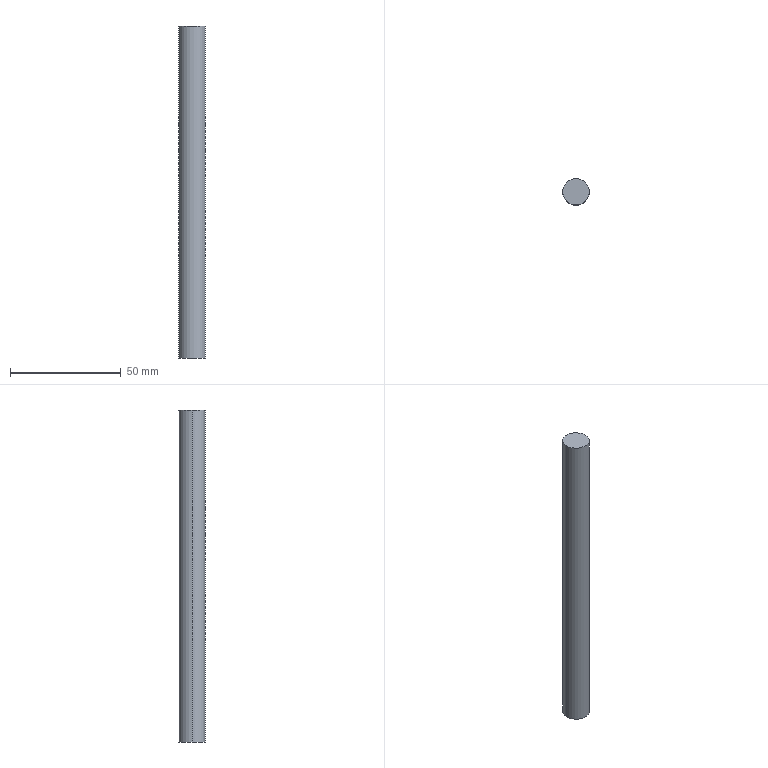Part | SolidWorks | features Extrusion 1 | 1 solid | 4 faces | box 12 x 12 x 150 mm | volume 16965 mm3 | cylinder 2 | plane 2 | commonest cylinder face diameters 12 x2
STEP:
#1=CARTESIAN_POINT('',(6.,0.,75.));
#2=VERTEX_POINT('',#1);
#3=CARTESIAN_POINT('',(-6.,0.,75.));
#4=VERTEX_POINT('',#3);
#5=CARTESIAN_POINT('',(0.,0.,75.));
#6=DIRECTION('',(0.,0.,1.));
#7=DIRECTION('',(1.,0.,0.));
#8=AXIS2_PLACEMENT_3D('',#5,#6,#7);
#9=CIRCLE('',#8,6.);
#10=EDGE_CURVE('',#2,#4,#9,.T.);
#11=ORIENTED_EDGE('',*,*,#10,.F.);
#12=CARTESIAN_POINT('',(6.,0.,-75.));
#13=VERTEX_POINT('',#12);
#14=CARTESIAN_POINT('',(6.,0.,75.));
#15=DIRECTION('',(0.,0.,-1.));
#16=VECTOR('',#15,1000.);
#17=LINE('',#14,#16);
#18=EDGE_CURVE('',#2,#13,#17,.T.);
#19=ORIENTED_EDGE('',*,*,#18,.T.);
#20=CARTESIAN_POINT('',(-6.,0.,-75.));
#21=VERTEX_POINT('',#20);
#22=CARTESIAN_POINT('',(0.,0.,-75.));
#23=DIRECTION('',(0.,0.,1.));
#24=DIRECTION('',(1.,0.,0.));
#25=AXIS2_PLACEMENT_3D('',#22,#23,#24);
#26=CIRCLE('',#25,6.);
#27=EDGE_CURVE('',#13,#21,#26,.T.);
#28=ORIENTED_EDGE('',*,*,#27,.T.);
#29=CARTESIAN_POINT('',(-6.,0.,75.));
#30=DIRECTION('',(0.,0.,-1.));
#31=VECTOR('',#30,1000.);
#32=LINE('',#29,#31);
#33=EDGE_CURVE('',#4,#21,#32,.T.);
#34=ORIENTED_EDGE('',*,*,#33,.F.);
#35=EDGE_LOOP('',(#11,#19,#28,#34));
#36=FACE_OUTER_BOUND('',#35,.T.);
#37=CARTESIAN_POINT('',(0.,0.,75.));
#38=DIRECTION('',(0.,0.,-1.));
#39=DIRECTION('',(-1.,0.,0.));
#40=AXIS2_PLACEMENT_3D('',#37,#38,#39);
#41=CYLINDRICAL_SURFACE('',#40,6.);
#42=ADVANCED_FACE('',(#36),#41,.T.);
#43=ORIENTED_EDGE('',*,*,#18,.F.);
#44=CARTESIAN_POINT('',(0.,0.,75.));
#45=DIRECTION('',(0.,0.,1.));
#46=DIRECTION('',(1.,0.,0.));
#47=AXIS2_PLACEMENT_3D('',#44,#45,#46);
#48=CIRCLE('',#47,6.);
#49=EDGE_CURVE('',#4,#2,#48,.T.);
#50=ORIENTED_EDGE('',*,*,#49,.F.);
#51=ORIENTED_EDGE('',*,*,#33,.T.);
#52=CARTESIAN_POINT('',(0.,0.,-75.));
#53=DIRECTION('',(0.,0.,1.));
#54=DIRECTION('',(1.,0.,0.));
#55=AXIS2_PLACEMENT_3D('',#52,#53,#54);
#56=CIRCLE('',#55,6.);
#57=EDGE_CURVE('',#21,#13,#56,.T.);
#58=ORIENTED_EDGE('',*,*,#57,.T.);
#59=EDGE_LOOP('',(#43,#50,#51,#58));
#60=FACE_OUTER_BOUND('',#59,.T.);
#61=CARTESIAN_POINT('',(0.,0.,75.));
#62=DIRECTION('',(0.,0.,-1.));
#63=DIRECTION('',(-1.,0.,0.));
#64=AXIS2_PLACEMENT_3D('',#61,#62,#63);
#65=CYLINDRICAL_SURFACE('',#64,6.);
#66=ADVANCED_FACE('',(#60),#65,.T.);
#67=ORIENTED_EDGE('',*,*,#49,.T.);
#68=ORIENTED_EDGE('',*,*,#10,.T.);
#69=EDGE_LOOP('',(#67,#68));
#70=FACE_OUTER_BOUND('',#69,.T.);
#71=CARTESIAN_POINT('',(0.,0.,75.));
#72=DIRECTION('',(0.,0.,1.));
#73=DIRECTION('',(1.,0.,0.));
#74=AXIS2_PLACEMENT_3D('',#71,#72,#73);
#75=PLANE('',#74);
#76=ADVANCED_FACE('',(#70),#75,.T.);
#77=ORIENTED_EDGE('',*,*,#57,.F.);
#78=ORIENTED_EDGE('',*,*,#27,.F.);
#79=EDGE_LOOP('',(#77,#78));
#80=FACE_OUTER_BOUND('',#79,.T.);
#81=CARTESIAN_POINT('',(0.,0.,-75.));
#82=DIRECTION('',(0.,0.,1.));
#83=DIRECTION('',(1.,0.,0.));
#84=AXIS2_PLACEMENT_3D('',#81,#82,#83);
#85=PLANE('',#84);
#86=ADVANCED_FACE('',(#80),#85,.F.);
#87=CLOSED_SHELL('',(#42,#66,#76,#86));
#88=MANIFOLD_SOLID_BREP('',#87);
#89=CARTESIAN_POINT('',(0.,0.,0.));
#90=DIRECTION('',(0.,0.,1.));
#91=DIRECTION('',(1.,0.,0.));
#92=AXIS2_PLACEMENT_3D('',#89,#90,#91);
#93=(LENGTH_UNIT()NAMED_UNIT(*)SI_UNIT(.MILLI.,.METRE.));
#94=UNCERTAINTY_MEASURE_WITH_UNIT(LENGTH_MEASURE(0.00001),#93,'','');
#95=(NAMED_UNIT(*)PLANE_ANGLE_UNIT()SI_UNIT($,.RADIAN.));
#96=(NAMED_UNIT(*)SI_UNIT($,.STERADIAN.)SOLID_ANGLE_UNIT());
#97=(GEOMETRIC_REPRESENTATION_CONTEXT(3)GLOBAL_UNCERTAINTY_ASSIGNED_CONTEXT((#94))GLOBAL_UNIT_ASSIGNED_CONTEXT((#93,#95,#96))REPRESENTATION_CONTEXT('',''));
#98=ADVANCED_BREP_SHAPE_REPRESENTATION('',(#88,#92),#97);